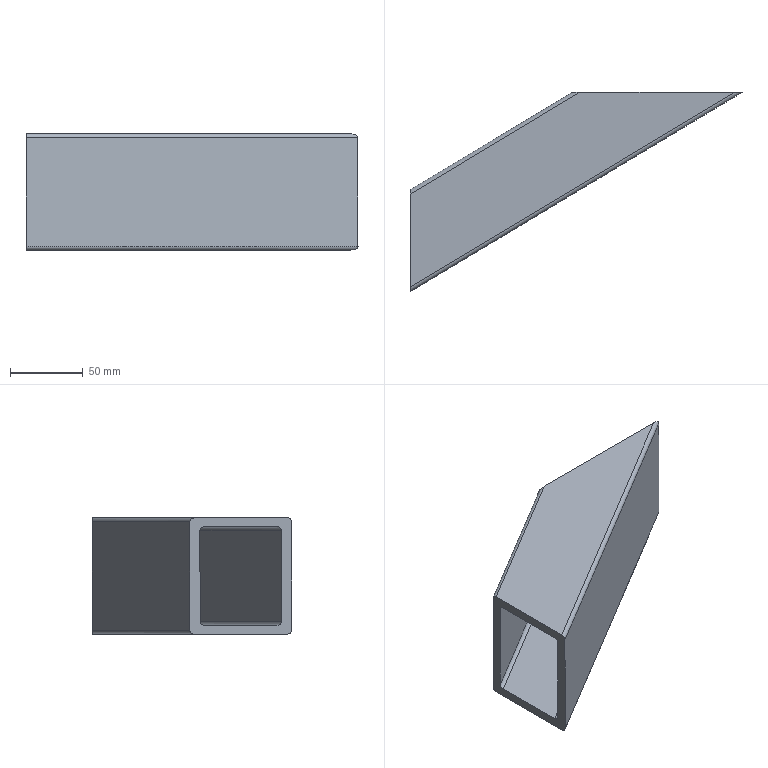Part | NX | 1 solid | 18 faces | box 228.355 x 137.013 x 80.035 mm | volume 304516 mm3 | plane 10 | cylinder 8 | commonest cylinder face diameters 5.236 x8
STEP:
#1=CARTESIAN_POINT('',(746.,374.988,-31.367));
#2=VERTEX_POINT('',#1);
#3=CARTESIAN_POINT('',(746.,375.035,31.397));
#4=VERTEX_POINT('',#3);
#5=CARTESIAN_POINT('',(746.,374.988,-31.375));
#6=DIRECTION('',(0.,0.0007377,1.));
#7=VECTOR('',#6,1000.);
#8=LINE('',#5,#7);
#9=EDGE_CURVE('',#2,#4,#8,.T.);
#10=ORIENTED_EDGE('',*,*,#9,.F.);
#11=CARTESIAN_POINT('',(746.,378.039,-33.986));
#12=VERTEX_POINT('',#11);
#13=CARTESIAN_POINT('',(746.,378.041,-31.368));
#14=DIRECTION('',(-1.,0.,0.));
#15=DIRECTION('',(0.,1.,0.));
#16=AXIS2_PLACEMENT_3D('',#13,#14,#15);
#17=ELLIPSE('',#16,3.053,2.618);
#18=EDGE_CURVE('',#12,#2,#17,.T.);
#19=ORIENTED_EDGE('',*,*,#18,.F.);
#20=CARTESIAN_POINT('',(746.,427.91,-34.014));
#21=VERTEX_POINT('',#20);
#22=CARTESIAN_POINT('',(746.,366.647,-33.98));
#23=DIRECTION('',(0.,-1.,0.0005424));
#24=VECTOR('',#23,1000.);
#25=LINE('',#22,#24);
#26=EDGE_CURVE('',#21,#12,#25,.T.);
#27=ORIENTED_EDGE('',*,*,#26,.F.);
#28=CARTESIAN_POINT('',(746.,430.965,-31.397));
#29=VERTEX_POINT('',#28);
#30=CARTESIAN_POINT('',(746.,427.912,-31.396));
#31=DIRECTION('',(-1.,0.,0.));
#32=DIRECTION('',(0.,1.,0.));
#33=AXIS2_PLACEMENT_3D('',#30,#31,#32);
#34=ELLIPSE('',#33,3.053,2.618);
#35=EDGE_CURVE('',#29,#21,#34,.T.);
#36=ORIENTED_EDGE('',*,*,#35,.F.);
#37=CARTESIAN_POINT('',(746.,431.012,31.367));
#38=VERTEX_POINT('',#37);
#39=CARTESIAN_POINT('',(746.,430.965,-31.416));
#40=DIRECTION('',(0.,-0.0007377,-1.));
#41=VECTOR('',#40,1000.);
#42=LINE('',#39,#41);
#43=EDGE_CURVE('',#38,#29,#42,.T.);
#44=ORIENTED_EDGE('',*,*,#43,.F.);
#45=CARTESIAN_POINT('',(746.,427.961,33.986));
#46=VERTEX_POINT('',#45);
#47=CARTESIAN_POINT('',(746.,427.959,31.368));
#48=DIRECTION('',(-1.,0.,0.));
#49=DIRECTION('',(0.,1.,0.));
#50=AXIS2_PLACEMENT_3D('',#47,#48,#49);
#51=ELLIPSE('',#50,3.053,2.618);
#52=EDGE_CURVE('',#46,#38,#51,.T.);
#53=ORIENTED_EDGE('',*,*,#52,.F.);
#54=CARTESIAN_POINT('',(746.,378.09,34.014));
#55=VERTEX_POINT('',#54);
#56=CARTESIAN_POINT('',(746.,366.684,34.02));
#57=DIRECTION('',(0.,1.,-0.0005424));
#58=VECTOR('',#57,1000.);
#59=LINE('',#56,#58);
#60=EDGE_CURVE('',#55,#46,#59,.T.);
#61=ORIENTED_EDGE('',*,*,#60,.F.);
#62=CARTESIAN_POINT('',(746.,378.088,31.396));
#63=DIRECTION('',(-1.,0.,0.));
#64=DIRECTION('',(0.,1.,0.));
#65=AXIS2_PLACEMENT_3D('',#62,#63,#64);
#66=ELLIPSE('',#65,3.053,2.618);
#67=EDGE_CURVE('',#4,#55,#66,.T.);
#68=ORIENTED_EDGE('',*,*,#67,.F.);
#69=EDGE_LOOP('',(#10,#19,#27,#36,#44,#53,#61,#68));
#70=FACE_BOUND('',#69,.T.);
#71=CARTESIAN_POINT('',(746.,434.903,-40.017));
#72=VERTEX_POINT('',#71);
#73=CARTESIAN_POINT('',(746.,371.038,-39.983));
#74=VERTEX_POINT('',#73);
#75=CARTESIAN_POINT('',(746.,361.498,-39.977));
#76=DIRECTION('',(0.,-1.,0.0005424));
#77=VECTOR('',#76,1000.);
#78=LINE('',#75,#77);
#79=EDGE_CURVE('',#72,#74,#78,.T.);
#80=ORIENTED_EDGE('',*,*,#79,.T.);
#81=CARTESIAN_POINT('',(746.,367.987,-37.363));
#82=VERTEX_POINT('',#81);
#83=CARTESIAN_POINT('',(746.,371.04,-37.365));
#84=DIRECTION('',(-1.,0.,0.));
#85=DIRECTION('',(0.,1.,0.));
#86=AXIS2_PLACEMENT_3D('',#83,#84,#85);
#87=ELLIPSE('',#86,3.053,2.618);
#88=EDGE_CURVE('',#74,#82,#87,.T.);
#89=ORIENTED_EDGE('',*,*,#88,.T.);
#90=CARTESIAN_POINT('',(746.,368.042,37.401));
#91=VERTEX_POINT('',#90);
#92=CARTESIAN_POINT('',(746.,367.987,-37.369));
#93=DIRECTION('',(0.,0.0007377,1.));
#94=VECTOR('',#93,1000.);
#95=LINE('',#92,#94);
#96=EDGE_CURVE('',#82,#91,#95,.T.);
#97=ORIENTED_EDGE('',*,*,#96,.T.);
#98=CARTESIAN_POINT('',(746.,371.097,40.017));
#99=VERTEX_POINT('',#98);
#100=CARTESIAN_POINT('',(746.,371.095,37.399));
#101=DIRECTION('',(-1.,0.,0.));
#102=DIRECTION('',(0.,1.,0.));
#103=AXIS2_PLACEMENT_3D('',#100,#101,#102);
#104=ELLIPSE('',#103,3.053,2.618);
#105=EDGE_CURVE('',#91,#99,#104,.T.);
#106=ORIENTED_EDGE('',*,*,#105,.T.);
#107=CARTESIAN_POINT('',(746.,434.962,39.983));
#108=VERTEX_POINT('',#107);
#109=CARTESIAN_POINT('',(746.,361.542,40.022));
#110=DIRECTION('',(0.,1.,-0.0005424));
#111=VECTOR('',#110,1000.);
#112=LINE('',#109,#111);
#113=EDGE_CURVE('',#99,#108,#112,.T.);
#114=ORIENTED_EDGE('',*,*,#113,.T.);
#115=CARTESIAN_POINT('',(746.,438.013,37.363));
#116=VERTEX_POINT('',#115);
#117=CARTESIAN_POINT('',(746.,434.96,37.365));
#118=DIRECTION('',(-1.,0.,0.));
#119=DIRECTION('',(0.,1.,0.));
#120=AXIS2_PLACEMENT_3D('',#117,#118,#119);
#121=ELLIPSE('',#120,3.053,2.618);
#122=EDGE_CURVE('',#108,#116,#121,.T.);
#123=ORIENTED_EDGE('',*,*,#122,.T.);
#124=CARTESIAN_POINT('',(746.,437.958,-37.401));
#125=VERTEX_POINT('',#124);
#126=CARTESIAN_POINT('',(746.,437.958,-37.421));
#127=DIRECTION('',(0.,-0.0007377,-1.));
#128=VECTOR('',#127,1000.);
#129=LINE('',#126,#128);
#130=EDGE_CURVE('',#116,#125,#129,.T.);
#131=ORIENTED_EDGE('',*,*,#130,.T.);
#132=CARTESIAN_POINT('',(746.,434.905,-37.399));
#133=DIRECTION('',(-1.,0.,0.));
#134=DIRECTION('',(0.,1.,0.));
#135=AXIS2_PLACEMENT_3D('',#132,#133,#134);
#136=ELLIPSE('',#135,3.053,2.618);
#137=EDGE_CURVE('',#125,#72,#136,.T.);
#138=ORIENTED_EDGE('',*,*,#137,.T.);
#139=EDGE_LOOP('',(#80,#89,#97,#106,#114,#123,#131,#138));
#140=FACE_BOUND('',#139,.T.);
#141=CARTESIAN_POINT('',(746.,535.,-37.382));
#142=DIRECTION('',(-1.,0.,0.));
#143=DIRECTION('',(0.,0.,1.));
#144=AXIS2_PLACEMENT_3D('',#141,#142,#143);
#145=PLANE('',#144);
#146=ADVANCED_FACE('',(#70,#140),#145,.T.);
#147=CARTESIAN_POINT('',(857.645,505.,37.363));
#148=VERTEX_POINT('',#147);
#149=CARTESIAN_POINT('',(862.73,505.,39.983));
#150=VERTEX_POINT('',#149);
#151=CARTESIAN_POINT('',(862.733,505.,37.365));
#152=DIRECTION('',(0.,1.,0.));
#153=DIRECTION('',(1.,0.,0.));
#154=AXIS2_PLACEMENT_3D('',#151,#152,#153);
#155=ELLIPSE('',#154,5.088,2.618);
#156=EDGE_CURVE('',#148,#150,#155,.T.);
#157=ORIENTED_EDGE('',*,*,#156,.F.);
#158=CARTESIAN_POINT('',(700.553,410.745,37.363));
#159=DIRECTION('',(0.8575,0.5145,0.));
#160=VECTOR('',#159,1000.);
#161=LINE('',#158,#160);
#162=EDGE_CURVE('',#116,#148,#161,.T.);
#163=ORIENTED_EDGE('',*,*,#162,.F.);
#164=ORIENTED_EDGE('',*,*,#122,.F.);
#165=CARTESIAN_POINT('',(701.899,408.502,39.983));
#166=DIRECTION('',(0.8575,0.5145,0.));
#167=VECTOR('',#166,1000.);
#168=LINE('',#165,#167);
#169=EDGE_CURVE('',#108,#150,#168,.T.);
#170=ORIENTED_EDGE('',*,*,#169,.T.);
#171=EDGE_LOOP('',(#157,#163,#164,#170));
#172=FACE_BOUND('',#171,.T.);
#173=CARTESIAN_POINT('',(701.9,408.5,37.365));
#174=DIRECTION('',(0.8575,0.5145,0.));
#175=DIRECTION('',(-0.5145,0.8575,0.));
#176=AXIS2_PLACEMENT_3D('',#173,#174,#175);
#177=CYLINDRICAL_SURFACE('',#176,2.618);
#178=ADVANCED_FACE('',(#172),#177,.T.);
#179=CARTESIAN_POINT('',(857.736,505.,-37.401));
#180=VERTEX_POINT('',#179);
#181=CARTESIAN_POINT('',(857.736,505.,-37.208));
#182=DIRECTION('',(-0.001229,0.,1.));
#183=VECTOR('',#182,1000.);
#184=LINE('',#181,#183);
#185=EDGE_CURVE('',#180,#148,#184,.T.);
#186=ORIENTED_EDGE('',*,*,#185,.F.);
#187=CARTESIAN_POINT('',(700.577,410.705,-37.401));
#188=DIRECTION('',(0.8575,0.5145,0.));
#189=VECTOR('',#188,1000.);
#190=LINE('',#187,#189);
#191=EDGE_CURVE('',#125,#180,#190,.T.);
#192=ORIENTED_EDGE('',*,*,#191,.F.);
#193=ORIENTED_EDGE('',*,*,#130,.F.);
#194=ORIENTED_EDGE('',*,*,#162,.T.);
#195=EDGE_LOOP('',(#186,#192,#193,#194));
#196=FACE_BOUND('',#195,.T.);
#197=CARTESIAN_POINT('',(700.577,410.705,-37.401));
#198=DIRECTION('',(0.5145,-0.8575,0.0006326));
#199=DIRECTION('',(0.8575,0.5145,0.));
#200=AXIS2_PLACEMENT_3D('',#197,#198,#199);
#201=PLANE('',#200);
#202=ADVANCED_FACE('',(#196),#201,.F.);
#203=CARTESIAN_POINT('',(974.355,505.,-37.363));
#204=VERTEX_POINT('',#203);
#205=CARTESIAN_POINT('',(969.27,505.,-39.983));
#206=VERTEX_POINT('',#205);
#207=CARTESIAN_POINT('',(969.267,505.,-37.365));
#208=DIRECTION('',(0.,1.,0.));
#209=DIRECTION('',(1.,0.,0.));
#210=AXIS2_PLACEMENT_3D('',#207,#208,#209);
#211=ELLIPSE('',#210,5.088,2.618);
#212=EDGE_CURVE('',#204,#206,#211,.T.);
#213=ORIENTED_EDGE('',*,*,#212,.F.);
#214=CARTESIAN_POINT('',(731.447,359.255,-37.363));
#215=DIRECTION('',(0.8575,0.5145,0.));
#216=VECTOR('',#215,1000.);
#217=LINE('',#214,#216);
#218=EDGE_CURVE('',#82,#204,#217,.T.);
#219=ORIENTED_EDGE('',*,*,#218,.F.);
#220=ORIENTED_EDGE('',*,*,#88,.F.);
#221=CARTESIAN_POINT('',(730.101,361.498,-39.983));
#222=DIRECTION('',(0.8575,0.5145,0.));
#223=VECTOR('',#222,1000.);
#224=LINE('',#221,#223);
#225=EDGE_CURVE('',#74,#206,#224,.T.);
#226=ORIENTED_EDGE('',*,*,#225,.T.);
#227=EDGE_LOOP('',(#213,#219,#220,#226));
#228=FACE_BOUND('',#227,.T.);
#229=CARTESIAN_POINT('',(730.1,361.5,-37.365));
#230=DIRECTION('',(0.8575,0.5145,0.));
#231=DIRECTION('',(-0.5145,0.8575,0.));
#232=AXIS2_PLACEMENT_3D('',#229,#230,#231);
#233=CYLINDRICAL_SURFACE('',#232,2.618);
#234=ADVANCED_FACE('',(#228),#233,.T.);
#235=CARTESIAN_POINT('',(974.264,505.,37.401));
#236=VERTEX_POINT('',#235);
#237=CARTESIAN_POINT('',(974.355,505.,-37.064));
#238=DIRECTION('',(0.001229,0.,-1.));
#239=VECTOR('',#238,1000.);
#240=LINE('',#237,#239);
#241=EDGE_CURVE('',#236,#204,#240,.T.);
#242=ORIENTED_EDGE('',*,*,#241,.F.);
#243=CARTESIAN_POINT('',(731.423,359.295,37.401));
#244=DIRECTION('',(0.8575,0.5145,0.));
#245=VECTOR('',#244,1000.);
#246=LINE('',#243,#245);
#247=EDGE_CURVE('',#91,#236,#246,.T.);
#248=ORIENTED_EDGE('',*,*,#247,.F.);
#249=ORIENTED_EDGE('',*,*,#96,.F.);
#250=ORIENTED_EDGE('',*,*,#218,.T.);
#251=EDGE_LOOP('',(#242,#248,#249,#250));
#252=FACE_BOUND('',#251,.T.);
#253=CARTESIAN_POINT('',(731.447,359.255,-37.363));
#254=DIRECTION('',(-0.5145,0.8575,-0.0006326));
#255=DIRECTION('',(-0.8575,-0.5145,0.));
#256=AXIS2_PLACEMENT_3D('',#253,#254,#255);
#257=PLANE('',#256);
#258=ADVANCED_FACE('',(#252),#257,.F.);
#259=CARTESIAN_POINT('',(957.517,505.,34.014));
#260=VERTEX_POINT('',#259);
#261=CARTESIAN_POINT('',(726.99,366.684,34.014));
#262=DIRECTION('',(0.8575,0.5145,0.));
#263=VECTOR('',#262,1000.);
#264=LINE('',#261,#263);
#265=EDGE_CURVE('',#55,#260,#264,.T.);
#266=ORIENTED_EDGE('',*,*,#265,.T.);
#267=CARTESIAN_POINT('',(962.609,505.,31.397));
#268=VERTEX_POINT('',#267);
#269=CARTESIAN_POINT('',(957.521,505.,31.396));
#270=DIRECTION('',(0.,1.,0.));
#271=DIRECTION('',(1.,0.,0.));
#272=AXIS2_PLACEMENT_3D('',#269,#270,#271);
#273=ELLIPSE('',#272,5.088,2.618);
#274=EDGE_CURVE('',#260,#268,#273,.T.);
#275=ORIENTED_EDGE('',*,*,#274,.T.);
#276=CARTESIAN_POINT('',(728.338,364.437,31.397));
#277=DIRECTION('',(0.8575,0.5145,0.));
#278=VECTOR('',#277,1000.);
#279=LINE('',#276,#278);
#280=EDGE_CURVE('',#4,#268,#279,.T.);
#281=ORIENTED_EDGE('',*,*,#280,.F.);
#282=ORIENTED_EDGE('',*,*,#67,.T.);
#283=EDGE_LOOP('',(#266,#275,#281,#282));
#284=FACE_BOUND('',#283,.T.);
#285=CARTESIAN_POINT('',(726.991,366.682,31.396));
#286=DIRECTION('',(0.8575,0.5145,0.));
#287=DIRECTION('',(-0.5145,0.8575,0.));
#288=AXIS2_PLACEMENT_3D('',#285,#286,#287);
#289=CYLINDRICAL_SURFACE('',#288,2.618);
#290=ADVANCED_FACE('',(#284),#289,.F.);
#291=ORIENTED_EDGE('',*,*,#280,.T.);
#292=CARTESIAN_POINT('',(962.686,505.,-31.367));
#293=VERTEX_POINT('',#292);
#294=CARTESIAN_POINT('',(962.686,505.,-31.079));
#295=DIRECTION('',(0.001229,0.,-1.));
#296=VECTOR('',#295,1000.);
#297=LINE('',#294,#296);
#298=EDGE_CURVE('',#268,#293,#297,.T.);
#299=ORIENTED_EDGE('',*,*,#298,.T.);
#300=CARTESIAN_POINT('',(728.358,364.403,-31.367));
#301=DIRECTION('',(0.8575,0.5145,0.));
#302=VECTOR('',#301,1000.);
#303=LINE('',#300,#302);
#304=EDGE_CURVE('',#2,#293,#303,.T.);
#305=ORIENTED_EDGE('',*,*,#304,.F.);
#306=ORIENTED_EDGE('',*,*,#9,.T.);
#307=EDGE_LOOP('',(#291,#299,#305,#306));
#308=FACE_BOUND('',#307,.T.);
#309=CARTESIAN_POINT('',(728.358,364.403,-31.367));
#310=DIRECTION('',(-0.5145,0.8575,-0.0006326));
#311=DIRECTION('',(-0.8575,-0.5145,0.));
#312=AXIS2_PLACEMENT_3D('',#309,#310,#311);
#313=PLANE('',#312);
#314=ADVANCED_FACE('',(#308),#313,.T.);
#315=ORIENTED_EDGE('',*,*,#304,.T.);
#316=CARTESIAN_POINT('',(957.601,505.,-33.986));
#317=VERTEX_POINT('',#316);
#318=CARTESIAN_POINT('',(957.598,505.,-31.368));
#319=DIRECTION('',(0.,1.,0.));
#320=DIRECTION('',(1.,0.,0.));
#321=AXIS2_PLACEMENT_3D('',#318,#319,#320);
#322=ELLIPSE('',#321,5.088,2.618);
#323=EDGE_CURVE('',#293,#317,#322,.T.);
#324=ORIENTED_EDGE('',*,*,#323,.T.);
#325=CARTESIAN_POINT('',(727.012,366.647,-33.986));
#326=DIRECTION('',(0.8575,0.5145,0.));
#327=VECTOR('',#326,1000.);
#328=LINE('',#325,#327);
#329=EDGE_CURVE('',#12,#317,#328,.T.);
#330=ORIENTED_EDGE('',*,*,#329,.F.);
#331=ORIENTED_EDGE('',*,*,#18,.T.);
#332=EDGE_LOOP('',(#315,#324,#330,#331));
#333=FACE_BOUND('',#332,.T.);
#334=CARTESIAN_POINT('',(727.011,366.648,-31.368));
#335=DIRECTION('',(0.8575,0.5145,0.));
#336=DIRECTION('',(-0.5145,0.8575,0.));
#337=AXIS2_PLACEMENT_3D('',#334,#335,#336);
#338=CYLINDRICAL_SURFACE('',#337,2.618);
#339=ADVANCED_FACE('',(#333),#338,.F.);
#340=ORIENTED_EDGE('',*,*,#329,.T.);
#341=CARTESIAN_POINT('',(874.483,505.,-34.014));
#342=VERTEX_POINT('',#341);
#343=CARTESIAN_POINT('',(727.012,505.,-34.062));
#344=DIRECTION('',(-1.,0.,-0.0003255));
#345=VECTOR('',#344,1000.);
#346=LINE('',#343,#345);
#347=EDGE_CURVE('',#317,#342,#346,.T.);
#348=ORIENTED_EDGE('',*,*,#347,.T.);
#349=CARTESIAN_POINT('',(705.01,403.316,-34.014));
#350=DIRECTION('',(0.8575,0.5145,0.));
#351=VECTOR('',#350,1000.);
#352=LINE('',#349,#351);
#353=EDGE_CURVE('',#21,#342,#352,.T.);
#354=ORIENTED_EDGE('',*,*,#353,.F.);
#355=ORIENTED_EDGE('',*,*,#26,.T.);
#356=EDGE_LOOP('',(#340,#348,#354,#355));
#357=FACE_BOUND('',#356,.T.);
#358=CARTESIAN_POINT('',(727.012,366.647,-33.986));
#359=DIRECTION('',(-0.0003255,0.0005424,1.));
#360=DIRECTION('',(0.,-1.,0.0005424));
#361=AXIS2_PLACEMENT_3D('',#358,#359,#360);
#362=PLANE('',#361);
#363=ADVANCED_FACE('',(#357),#362,.T.);
#364=ORIENTED_EDGE('',*,*,#353,.T.);
#365=CARTESIAN_POINT('',(869.391,505.,-31.397));
#366=VERTEX_POINT('',#365);
#367=CARTESIAN_POINT('',(874.479,505.,-31.396));
#368=DIRECTION('',(0.,1.,0.));
#369=DIRECTION('',(1.,0.,0.));
#370=AXIS2_PLACEMENT_3D('',#367,#368,#369);
#371=ELLIPSE('',#370,5.088,2.618);
#372=EDGE_CURVE('',#342,#366,#371,.T.);
#373=ORIENTED_EDGE('',*,*,#372,.T.);
#374=CARTESIAN_POINT('',(703.662,405.563,-31.397));
#375=DIRECTION('',(0.8575,0.5145,0.));
#376=VECTOR('',#375,1000.);
#377=LINE('',#374,#376);
#378=EDGE_CURVE('',#29,#366,#377,.T.);
#379=ORIENTED_EDGE('',*,*,#378,.F.);
#380=ORIENTED_EDGE('',*,*,#35,.T.);
#381=EDGE_LOOP('',(#364,#373,#379,#380));
#382=FACE_BOUND('',#381,.T.);
#383=CARTESIAN_POINT('',(705.009,403.318,-31.396));
#384=DIRECTION('',(0.8575,0.5145,0.));
#385=DIRECTION('',(-0.5145,0.8575,0.));
#386=AXIS2_PLACEMENT_3D('',#383,#384,#385);
#387=CYLINDRICAL_SURFACE('',#386,2.618);
#388=ADVANCED_FACE('',(#382),#387,.F.);
#389=ORIENTED_EDGE('',*,*,#378,.T.);
#390=CARTESIAN_POINT('',(869.314,505.,31.367));
#391=VERTEX_POINT('',#390);
#392=CARTESIAN_POINT('',(869.391,505.,-31.193));
#393=DIRECTION('',(-0.001229,0.,1.));
#394=VECTOR('',#393,1000.);
#395=LINE('',#392,#394);
#396=EDGE_CURVE('',#366,#391,#395,.T.);
#397=ORIENTED_EDGE('',*,*,#396,.T.);
#398=CARTESIAN_POINT('',(703.642,405.597,31.367));
#399=DIRECTION('',(0.8575,0.5145,0.));
#400=VECTOR('',#399,1000.);
#401=LINE('',#398,#400);
#402=EDGE_CURVE('',#38,#391,#401,.T.);
#403=ORIENTED_EDGE('',*,*,#402,.F.);
#404=ORIENTED_EDGE('',*,*,#43,.T.);
#405=EDGE_LOOP('',(#389,#397,#403,#404));
#406=FACE_BOUND('',#405,.T.);
#407=CARTESIAN_POINT('',(703.662,405.563,-31.397));
#408=DIRECTION('',(0.5145,-0.8575,0.0006326));
#409=DIRECTION('',(0.8575,0.5145,0.));
#410=AXIS2_PLACEMENT_3D('',#407,#408,#409);
#411=PLANE('',#410);
#412=ADVANCED_FACE('',(#406),#411,.T.);
#413=ORIENTED_EDGE('',*,*,#402,.T.);
#414=CARTESIAN_POINT('',(874.399,505.,33.986));
#415=VERTEX_POINT('',#414);
#416=CARTESIAN_POINT('',(874.402,505.,31.368));
#417=DIRECTION('',(0.,1.,0.));
#418=DIRECTION('',(1.,0.,0.));
#419=AXIS2_PLACEMENT_3D('',#416,#417,#418);
#420=ELLIPSE('',#419,5.088,2.618);
#421=EDGE_CURVE('',#391,#415,#420,.T.);
#422=ORIENTED_EDGE('',*,*,#421,.T.);
#423=CARTESIAN_POINT('',(704.988,403.353,33.986));
#424=DIRECTION('',(0.8575,0.5145,0.));
#425=VECTOR('',#424,1000.);
#426=LINE('',#423,#425);
#427=EDGE_CURVE('',#46,#415,#426,.T.);
#428=ORIENTED_EDGE('',*,*,#427,.F.);
#429=ORIENTED_EDGE('',*,*,#52,.T.);
#430=EDGE_LOOP('',(#413,#422,#428,#429));
#431=FACE_BOUND('',#430,.T.);
#432=CARTESIAN_POINT('',(704.989,403.352,31.368));
#433=DIRECTION('',(0.8575,0.5145,0.));
#434=DIRECTION('',(-0.5145,0.8575,0.));
#435=AXIS2_PLACEMENT_3D('',#432,#433,#434);
#436=CYLINDRICAL_SURFACE('',#435,2.618);
#437=ADVANCED_FACE('',(#431),#436,.F.);
#438=ORIENTED_EDGE('',*,*,#427,.T.);
#439=CARTESIAN_POINT('',(726.99,505.,33.938));
#440=DIRECTION('',(1.,0.,0.0003255));
#441=VECTOR('',#440,1000.);
#442=LINE('',#439,#441);
#443=EDGE_CURVE('',#415,#260,#442,.T.);
#444=ORIENTED_EDGE('',*,*,#443,.T.);
#445=ORIENTED_EDGE('',*,*,#265,.F.);
#446=ORIENTED_EDGE('',*,*,#60,.T.);
#447=EDGE_LOOP('',(#438,#444,#445,#446));
#448=FACE_BOUND('',#447,.T.);
#449=CARTESIAN_POINT('',(726.99,366.684,34.014));
#450=DIRECTION('',(0.0003255,-0.0005424,-1.));
#451=DIRECTION('',(0.,1.,-0.0005424));
#452=AXIS2_PLACEMENT_3D('',#449,#450,#451);
#453=PLANE('',#452);
#454=ADVANCED_FACE('',(#448),#453,.T.);
#455=ORIENTED_EDGE('',*,*,#443,.F.);
#456=ORIENTED_EDGE('',*,*,#421,.F.);
#457=ORIENTED_EDGE('',*,*,#396,.F.);
#458=ORIENTED_EDGE('',*,*,#372,.F.);
#459=ORIENTED_EDGE('',*,*,#347,.F.);
#460=ORIENTED_EDGE('',*,*,#323,.F.);
#461=ORIENTED_EDGE('',*,*,#298,.F.);
#462=ORIENTED_EDGE('',*,*,#274,.F.);
#463=EDGE_LOOP('',(#455,#456,#457,#458,#459,#460,#461,#462));
#464=FACE_BOUND('',#463,.T.);
#465=CARTESIAN_POINT('',(969.172,505.,40.017));
#466=VERTEX_POINT('',#465);
#467=CARTESIAN_POINT('',(969.175,505.,37.399));
#468=DIRECTION('',(0.,1.,0.));
#469=DIRECTION('',(1.,0.,0.));
#470=AXIS2_PLACEMENT_3D('',#467,#468,#469);
#471=ELLIPSE('',#470,5.088,2.618);
#472=EDGE_CURVE('',#466,#236,#471,.T.);
#473=ORIENTED_EDGE('',*,*,#472,.T.);
#474=ORIENTED_EDGE('',*,*,#241,.T.);
#475=ORIENTED_EDGE('',*,*,#212,.T.);
#476=CARTESIAN_POINT('',(862.828,505.,-40.017));
#477=VERTEX_POINT('',#476);
#478=CARTESIAN_POINT('',(730.101,505.,-40.061));
#479=DIRECTION('',(-1.,0.,-0.0003255));
#480=VECTOR('',#479,1000.);
#481=LINE('',#478,#480);
#482=EDGE_CURVE('',#206,#477,#481,.T.);
#483=ORIENTED_EDGE('',*,*,#482,.T.);
#484=CARTESIAN_POINT('',(862.825,505.,-37.399));
#485=DIRECTION('',(0.,1.,0.));
#486=DIRECTION('',(1.,0.,0.));
#487=AXIS2_PLACEMENT_3D('',#484,#485,#486);
#488=ELLIPSE('',#487,5.088,2.618);
#489=EDGE_CURVE('',#477,#180,#488,.T.);
#490=ORIENTED_EDGE('',*,*,#489,.T.);
#491=ORIENTED_EDGE('',*,*,#185,.T.);
#492=ORIENTED_EDGE('',*,*,#156,.T.);
#493=CARTESIAN_POINT('',(730.075,505.,39.939));
#494=DIRECTION('',(1.,0.,0.0003255));
#495=VECTOR('',#494,1000.);
#496=LINE('',#493,#495);
#497=EDGE_CURVE('',#150,#466,#496,.T.);
#498=ORIENTED_EDGE('',*,*,#497,.T.);
#499=EDGE_LOOP('',(#473,#474,#475,#483,#490,#491,#492,#498));
#500=FACE_BOUND('',#499,.T.);
#501=CARTESIAN_POINT('',(1126.,505.,37.382));
#502=DIRECTION('',(0.,1.,0.));
#503=DIRECTION('',(0.,0.,1.));
#504=AXIS2_PLACEMENT_3D('',#501,#502,#503);
#505=PLANE('',#504);
#506=ADVANCED_FACE('',(#464,#500),#505,.T.);
#507=ORIENTED_EDGE('',*,*,#489,.F.);
#508=CARTESIAN_POINT('',(701.925,408.458,-40.017));
#509=DIRECTION('',(0.8575,0.5145,0.));
#510=VECTOR('',#509,1000.);
#511=LINE('',#508,#510);
#512=EDGE_CURVE('',#72,#477,#511,.T.);
#513=ORIENTED_EDGE('',*,*,#512,.F.);
#514=ORIENTED_EDGE('',*,*,#137,.F.);
#515=ORIENTED_EDGE('',*,*,#191,.T.);
#516=EDGE_LOOP('',(#507,#513,#514,#515));
#517=FACE_BOUND('',#516,.T.);
#518=CARTESIAN_POINT('',(701.924,408.46,-37.399));
#519=DIRECTION('',(0.8575,0.5145,0.));
#520=DIRECTION('',(-0.5145,0.8575,0.));
#521=AXIS2_PLACEMENT_3D('',#518,#519,#520);
#522=CYLINDRICAL_SURFACE('',#521,2.618);
#523=ADVANCED_FACE('',(#517),#522,.T.);
#524=ORIENTED_EDGE('',*,*,#512,.T.);
#525=ORIENTED_EDGE('',*,*,#482,.F.);
#526=ORIENTED_EDGE('',*,*,#225,.F.);
#527=ORIENTED_EDGE('',*,*,#79,.F.);
#528=EDGE_LOOP('',(#524,#525,#526,#527));
#529=FACE_BOUND('',#528,.T.);
#530=CARTESIAN_POINT('',(730.101,361.498,-39.983));
#531=DIRECTION('',(-0.0003255,0.0005424,1.));
#532=DIRECTION('',(0.,-1.,0.0005424));
#533=AXIS2_PLACEMENT_3D('',#530,#531,#532);
#534=PLANE('',#533);
#535=ADVANCED_FACE('',(#529),#534,.F.);
#536=ORIENTED_EDGE('',*,*,#472,.F.);
#537=CARTESIAN_POINT('',(730.075,361.542,40.017));
#538=DIRECTION('',(0.8575,0.5145,0.));
#539=VECTOR('',#538,1000.);
#540=LINE('',#537,#539);
#541=EDGE_CURVE('',#99,#466,#540,.T.);
#542=ORIENTED_EDGE('',*,*,#541,.F.);
#543=ORIENTED_EDGE('',*,*,#105,.F.);
#544=ORIENTED_EDGE('',*,*,#247,.T.);
#545=EDGE_LOOP('',(#536,#542,#543,#544));
#546=FACE_BOUND('',#545,.T.);
#547=CARTESIAN_POINT('',(730.076,361.54,37.399));
#548=DIRECTION('',(0.8575,0.5145,0.));
#549=DIRECTION('',(-0.5145,0.8575,0.));
#550=AXIS2_PLACEMENT_3D('',#547,#548,#549);
#551=CYLINDRICAL_SURFACE('',#550,2.618);
#552=ADVANCED_FACE('',(#546),#551,.T.);
#553=ORIENTED_EDGE('',*,*,#541,.T.);
#554=ORIENTED_EDGE('',*,*,#497,.F.);
#555=ORIENTED_EDGE('',*,*,#169,.F.);
#556=ORIENTED_EDGE('',*,*,#113,.F.);
#557=EDGE_LOOP('',(#553,#554,#555,#556));
#558=FACE_BOUND('',#557,.T.);
#559=CARTESIAN_POINT('',(730.075,361.542,40.017));
#560=DIRECTION('',(0.0003255,-0.0005424,-1.));
#561=DIRECTION('',(0.,1.,-0.0005424));
#562=AXIS2_PLACEMENT_3D('',#559,#560,#561);
#563=PLANE('',#562);
#564=ADVANCED_FACE('',(#558),#563,.F.);
#565=CLOSED_SHELL('',(#146,#178,#202,#234,#258,#290,#314,#339,#363,#388,#412,#437,#454,#506,#523,#535,#552,#564));
#566=MANIFOLD_SOLID_BREP('',#565);
#567=(LENGTH_UNIT()NAMED_UNIT(*)SI_UNIT(.MILLI.,.METRE.));
#568=UNCERTAINTY_MEASURE_WITH_UNIT(LENGTH_MEASURE(0.00001),#567,'','');
#569=(NAMED_UNIT(*)PLANE_ANGLE_UNIT()SI_UNIT($,.RADIAN.));
#570=(NAMED_UNIT(*)SI_UNIT($,.STERADIAN.)SOLID_ANGLE_UNIT());
#571=(GEOMETRIC_REPRESENTATION_CONTEXT(3)GLOBAL_UNCERTAINTY_ASSIGNED_CONTEXT((#568))GLOBAL_UNIT_ASSIGNED_CONTEXT((#567,#569,#570))REPRESENTATION_CONTEXT('',''));
#572=ADVANCED_BREP_SHAPE_REPRESENTATION('',(#566),#571);